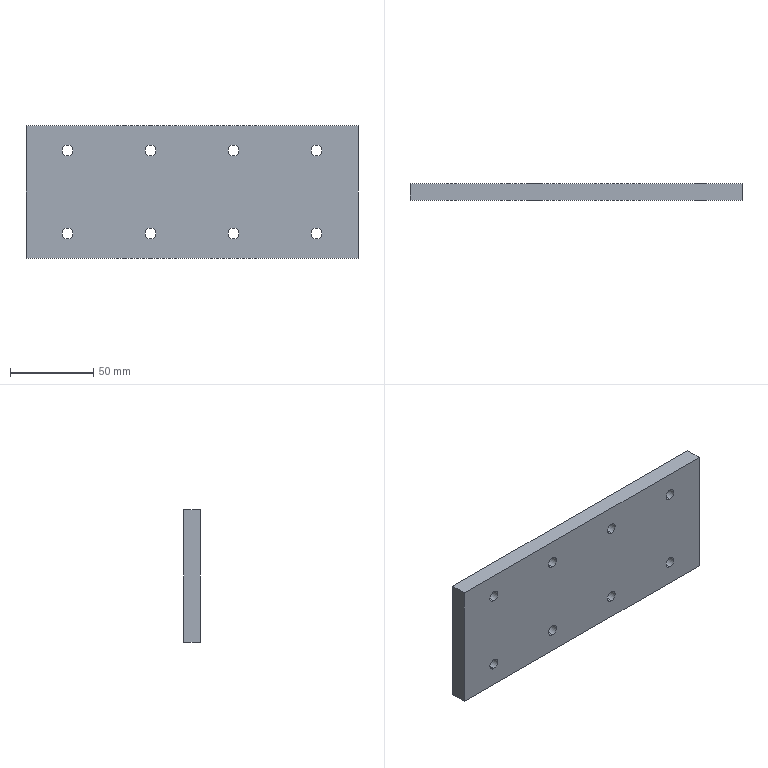Part | SolidWorks | features Extrusion 1, HoleWzd 1 | 1 solid | 22 faces | box 200 x 10 x 80 mm | volume 157263 mm3 | cylinder 16 | plane 6 | commonest cylinder face diameters 6.6 x16
STEP:
#1=CARTESIAN_POINT('',(-25.,0.,-28.3));
#2=VERTEX_POINT('',#1);
#3=CARTESIAN_POINT('',(-25.,0.,-21.7));
#4=VERTEX_POINT('',#3);
#5=CARTESIAN_POINT('',(-25.,0.,-25.));
#6=DIRECTION('',(0.,1.,0.));
#7=DIRECTION('',(0.,0.,1.));
#8=AXIS2_PLACEMENT_3D('',#5,#6,#7);
#9=CIRCLE('',#8,3.3);
#10=EDGE_CURVE('',#2,#4,#9,.T.);
#11=ORIENTED_EDGE('',*,*,#10,.F.);
#12=CARTESIAN_POINT('',(-25.,10.,-28.3));
#13=VERTEX_POINT('',#12);
#14=CARTESIAN_POINT('',(-25.,10.,-28.3));
#15=DIRECTION('',(0.,1.,0.));
#16=VECTOR('',#15,1000.);
#17=LINE('',#14,#16);
#18=EDGE_CURVE('',#2,#13,#17,.T.);
#19=ORIENTED_EDGE('',*,*,#18,.T.);
#20=CARTESIAN_POINT('',(-25.,10.,-21.7));
#21=VERTEX_POINT('',#20);
#22=CARTESIAN_POINT('',(-25.,10.,-25.));
#23=DIRECTION('',(0.,1.,0.));
#24=DIRECTION('',(0.,0.,1.));
#25=AXIS2_PLACEMENT_3D('',#22,#23,#24);
#26=CIRCLE('',#25,3.3);
#27=EDGE_CURVE('',#13,#21,#26,.T.);
#28=ORIENTED_EDGE('',*,*,#27,.T.);
#29=CARTESIAN_POINT('',(-25.,10.,-21.7));
#30=DIRECTION('',(0.,1.,0.));
#31=VECTOR('',#30,1000.);
#32=LINE('',#29,#31);
#33=EDGE_CURVE('',#4,#21,#32,.T.);
#34=ORIENTED_EDGE('',*,*,#33,.F.);
#35=EDGE_LOOP('',(#11,#19,#28,#34));
#36=FACE_OUTER_BOUND('',#35,.T.);
#37=CARTESIAN_POINT('',(-25.,10.,-25.));
#38=DIRECTION('',(0.,1.,0.));
#39=DIRECTION('',(0.,0.,1.));
#40=AXIS2_PLACEMENT_3D('',#37,#38,#39);
#41=CYLINDRICAL_SURFACE('',#40,3.3);
#42=ADVANCED_FACE('',(#36),#41,.F.);
#43=CARTESIAN_POINT('',(25.,0.,-28.3));
#44=VERTEX_POINT('',#43);
#45=CARTESIAN_POINT('',(25.,0.,-21.7));
#46=VERTEX_POINT('',#45);
#47=CARTESIAN_POINT('',(25.,0.,-25.));
#48=DIRECTION('',(0.,1.,0.));
#49=DIRECTION('',(0.,0.,1.));
#50=AXIS2_PLACEMENT_3D('',#47,#48,#49);
#51=CIRCLE('',#50,3.3);
#52=EDGE_CURVE('',#44,#46,#51,.T.);
#53=ORIENTED_EDGE('',*,*,#52,.F.);
#54=CARTESIAN_POINT('',(25.,10.,-28.3));
#55=VERTEX_POINT('',#54);
#56=CARTESIAN_POINT('',(25.,10.,-28.3));
#57=DIRECTION('',(0.,1.,0.));
#58=VECTOR('',#57,1000.);
#59=LINE('',#56,#58);
#60=EDGE_CURVE('',#44,#55,#59,.T.);
#61=ORIENTED_EDGE('',*,*,#60,.T.);
#62=CARTESIAN_POINT('',(25.,10.,-21.7));
#63=VERTEX_POINT('',#62);
#64=CARTESIAN_POINT('',(25.,10.,-25.));
#65=DIRECTION('',(0.,1.,0.));
#66=DIRECTION('',(0.,0.,1.));
#67=AXIS2_PLACEMENT_3D('',#64,#65,#66);
#68=CIRCLE('',#67,3.3);
#69=EDGE_CURVE('',#55,#63,#68,.T.);
#70=ORIENTED_EDGE('',*,*,#69,.T.);
#71=CARTESIAN_POINT('',(25.,10.,-21.7));
#72=DIRECTION('',(0.,1.,0.));
#73=VECTOR('',#72,1000.);
#74=LINE('',#71,#73);
#75=EDGE_CURVE('',#46,#63,#74,.T.);
#76=ORIENTED_EDGE('',*,*,#75,.F.);
#77=EDGE_LOOP('',(#53,#61,#70,#76));
#78=FACE_OUTER_BOUND('',#77,.T.);
#79=CARTESIAN_POINT('',(25.,10.,-25.));
#80=DIRECTION('',(0.,1.,0.));
#81=DIRECTION('',(0.,0.,1.));
#82=AXIS2_PLACEMENT_3D('',#79,#80,#81);
#83=CYLINDRICAL_SURFACE('',#82,3.3);
#84=ADVANCED_FACE('',(#78),#83,.F.);
#85=CARTESIAN_POINT('',(-25.,0.,21.7));
#86=VERTEX_POINT('',#85);
#87=CARTESIAN_POINT('',(-25.,0.,28.3));
#88=VERTEX_POINT('',#87);
#89=CARTESIAN_POINT('',(-25.,0.,25.));
#90=DIRECTION('',(0.,1.,0.));
#91=DIRECTION('',(0.,0.,1.));
#92=AXIS2_PLACEMENT_3D('',#89,#90,#91);
#93=CIRCLE('',#92,3.3);
#94=EDGE_CURVE('',#86,#88,#93,.T.);
#95=ORIENTED_EDGE('',*,*,#94,.F.);
#96=CARTESIAN_POINT('',(-25.,10.,21.7));
#97=VERTEX_POINT('',#96);
#98=CARTESIAN_POINT('',(-25.,10.,21.7));
#99=DIRECTION('',(0.,1.,0.));
#100=VECTOR('',#99,1000.);
#101=LINE('',#98,#100);
#102=EDGE_CURVE('',#86,#97,#101,.T.);
#103=ORIENTED_EDGE('',*,*,#102,.T.);
#104=CARTESIAN_POINT('',(-25.,10.,28.3));
#105=VERTEX_POINT('',#104);
#106=CARTESIAN_POINT('',(-25.,10.,25.));
#107=DIRECTION('',(0.,1.,0.));
#108=DIRECTION('',(0.,0.,1.));
#109=AXIS2_PLACEMENT_3D('',#106,#107,#108);
#110=CIRCLE('',#109,3.3);
#111=EDGE_CURVE('',#97,#105,#110,.T.);
#112=ORIENTED_EDGE('',*,*,#111,.T.);
#113=CARTESIAN_POINT('',(-25.,10.,28.3));
#114=DIRECTION('',(0.,1.,0.));
#115=VECTOR('',#114,1000.);
#116=LINE('',#113,#115);
#117=EDGE_CURVE('',#88,#105,#116,.T.);
#118=ORIENTED_EDGE('',*,*,#117,.F.);
#119=EDGE_LOOP('',(#95,#103,#112,#118));
#120=FACE_OUTER_BOUND('',#119,.T.);
#121=CARTESIAN_POINT('',(-25.,10.,25.));
#122=DIRECTION('',(0.,1.,0.));
#123=DIRECTION('',(0.,0.,1.));
#124=AXIS2_PLACEMENT_3D('',#121,#122,#123);
#125=CYLINDRICAL_SURFACE('',#124,3.3);
#126=ADVANCED_FACE('',(#120),#125,.F.);
#127=CARTESIAN_POINT('',(25.,0.,21.7));
#128=VERTEX_POINT('',#127);
#129=CARTESIAN_POINT('',(25.,0.,28.3));
#130=VERTEX_POINT('',#129);
#131=CARTESIAN_POINT('',(25.,0.,25.));
#132=DIRECTION('',(0.,1.,0.));
#133=DIRECTION('',(0.,0.,1.));
#134=AXIS2_PLACEMENT_3D('',#131,#132,#133);
#135=CIRCLE('',#134,3.3);
#136=EDGE_CURVE('',#128,#130,#135,.T.);
#137=ORIENTED_EDGE('',*,*,#136,.F.);
#138=CARTESIAN_POINT('',(25.,10.,21.7));
#139=VERTEX_POINT('',#138);
#140=CARTESIAN_POINT('',(25.,10.,21.7));
#141=DIRECTION('',(0.,1.,0.));
#142=VECTOR('',#141,1000.);
#143=LINE('',#140,#142);
#144=EDGE_CURVE('',#128,#139,#143,.T.);
#145=ORIENTED_EDGE('',*,*,#144,.T.);
#146=CARTESIAN_POINT('',(25.,10.,28.3));
#147=VERTEX_POINT('',#146);
#148=CARTESIAN_POINT('',(25.,10.,25.));
#149=DIRECTION('',(0.,1.,0.));
#150=DIRECTION('',(0.,0.,1.));
#151=AXIS2_PLACEMENT_3D('',#148,#149,#150);
#152=CIRCLE('',#151,3.3);
#153=EDGE_CURVE('',#139,#147,#152,.T.);
#154=ORIENTED_EDGE('',*,*,#153,.T.);
#155=CARTESIAN_POINT('',(25.,10.,28.3));
#156=DIRECTION('',(0.,1.,0.));
#157=VECTOR('',#156,1000.);
#158=LINE('',#155,#157);
#159=EDGE_CURVE('',#130,#147,#158,.T.);
#160=ORIENTED_EDGE('',*,*,#159,.F.);
#161=EDGE_LOOP('',(#137,#145,#154,#160));
#162=FACE_OUTER_BOUND('',#161,.T.);
#163=CARTESIAN_POINT('',(25.,10.,25.));
#164=DIRECTION('',(0.,1.,0.));
#165=DIRECTION('',(0.,0.,1.));
#166=AXIS2_PLACEMENT_3D('',#163,#164,#165);
#167=CYLINDRICAL_SURFACE('',#166,3.3);
#168=ADVANCED_FACE('',(#162),#167,.F.);
#169=CARTESIAN_POINT('',(-75.,0.,-28.3));
#170=VERTEX_POINT('',#169);
#171=CARTESIAN_POINT('',(-75.,0.,-21.7));
#172=VERTEX_POINT('',#171);
#173=CARTESIAN_POINT('',(-75.,0.,-25.));
#174=DIRECTION('',(0.,1.,0.));
#175=DIRECTION('',(0.,0.,1.));
#176=AXIS2_PLACEMENT_3D('',#173,#174,#175);
#177=CIRCLE('',#176,3.3);
#178=EDGE_CURVE('',#170,#172,#177,.T.);
#179=ORIENTED_EDGE('',*,*,#178,.F.);
#180=CARTESIAN_POINT('',(-75.,10.,-28.3));
#181=VERTEX_POINT('',#180);
#182=CARTESIAN_POINT('',(-75.,10.,-28.3));
#183=DIRECTION('',(0.,1.,0.));
#184=VECTOR('',#183,1000.);
#185=LINE('',#182,#184);
#186=EDGE_CURVE('',#170,#181,#185,.T.);
#187=ORIENTED_EDGE('',*,*,#186,.T.);
#188=CARTESIAN_POINT('',(-75.,10.,-21.7));
#189=VERTEX_POINT('',#188);
#190=CARTESIAN_POINT('',(-75.,10.,-25.));
#191=DIRECTION('',(0.,1.,0.));
#192=DIRECTION('',(0.,0.,1.));
#193=AXIS2_PLACEMENT_3D('',#190,#191,#192);
#194=CIRCLE('',#193,3.3);
#195=EDGE_CURVE('',#181,#189,#194,.T.);
#196=ORIENTED_EDGE('',*,*,#195,.T.);
#197=CARTESIAN_POINT('',(-75.,10.,-21.7));
#198=DIRECTION('',(0.,1.,0.));
#199=VECTOR('',#198,1000.);
#200=LINE('',#197,#199);
#201=EDGE_CURVE('',#172,#189,#200,.T.);
#202=ORIENTED_EDGE('',*,*,#201,.F.);
#203=EDGE_LOOP('',(#179,#187,#196,#202));
#204=FACE_OUTER_BOUND('',#203,.T.);
#205=CARTESIAN_POINT('',(-75.,10.,-25.));
#206=DIRECTION('',(0.,1.,0.));
#207=DIRECTION('',(0.,0.,1.));
#208=AXIS2_PLACEMENT_3D('',#205,#206,#207);
#209=CYLINDRICAL_SURFACE('',#208,3.3);
#210=ADVANCED_FACE('',(#204),#209,.F.);
#211=CARTESIAN_POINT('',(75.,0.,-28.3));
#212=VERTEX_POINT('',#211);
#213=CARTESIAN_POINT('',(75.,0.,-21.7));
#214=VERTEX_POINT('',#213);
#215=CARTESIAN_POINT('',(75.,0.,-25.));
#216=DIRECTION('',(0.,1.,0.));
#217=DIRECTION('',(0.,0.,1.));
#218=AXIS2_PLACEMENT_3D('',#215,#216,#217);
#219=CIRCLE('',#218,3.3);
#220=EDGE_CURVE('',#212,#214,#219,.T.);
#221=ORIENTED_EDGE('',*,*,#220,.F.);
#222=CARTESIAN_POINT('',(75.,10.,-28.3));
#223=VERTEX_POINT('',#222);
#224=CARTESIAN_POINT('',(75.,10.,-28.3));
#225=DIRECTION('',(0.,1.,0.));
#226=VECTOR('',#225,1000.);
#227=LINE('',#224,#226);
#228=EDGE_CURVE('',#212,#223,#227,.T.);
#229=ORIENTED_EDGE('',*,*,#228,.T.);
#230=CARTESIAN_POINT('',(75.,10.,-21.7));
#231=VERTEX_POINT('',#230);
#232=CARTESIAN_POINT('',(75.,10.,-25.));
#233=DIRECTION('',(0.,1.,0.));
#234=DIRECTION('',(0.,0.,1.));
#235=AXIS2_PLACEMENT_3D('',#232,#233,#234);
#236=CIRCLE('',#235,3.3);
#237=EDGE_CURVE('',#223,#231,#236,.T.);
#238=ORIENTED_EDGE('',*,*,#237,.T.);
#239=CARTESIAN_POINT('',(75.,10.,-21.7));
#240=DIRECTION('',(0.,1.,0.));
#241=VECTOR('',#240,1000.);
#242=LINE('',#239,#241);
#243=EDGE_CURVE('',#214,#231,#242,.T.);
#244=ORIENTED_EDGE('',*,*,#243,.F.);
#245=EDGE_LOOP('',(#221,#229,#238,#244));
#246=FACE_OUTER_BOUND('',#245,.T.);
#247=CARTESIAN_POINT('',(75.,10.,-25.));
#248=DIRECTION('',(0.,1.,0.));
#249=DIRECTION('',(0.,0.,1.));
#250=AXIS2_PLACEMENT_3D('',#247,#248,#249);
#251=CYLINDRICAL_SURFACE('',#250,3.3);
#252=ADVANCED_FACE('',(#246),#251,.F.);
#253=CARTESIAN_POINT('',(75.,0.,21.7));
#254=VERTEX_POINT('',#253);
#255=CARTESIAN_POINT('',(75.,0.,28.3));
#256=VERTEX_POINT('',#255);
#257=CARTESIAN_POINT('',(75.,0.,25.));
#258=DIRECTION('',(0.,1.,0.));
#259=DIRECTION('',(0.,0.,1.));
#260=AXIS2_PLACEMENT_3D('',#257,#258,#259);
#261=CIRCLE('',#260,3.3);
#262=EDGE_CURVE('',#254,#256,#261,.T.);
#263=ORIENTED_EDGE('',*,*,#262,.F.);
#264=CARTESIAN_POINT('',(75.,10.,21.7));
#265=VERTEX_POINT('',#264);
#266=CARTESIAN_POINT('',(75.,10.,21.7));
#267=DIRECTION('',(0.,1.,0.));
#268=VECTOR('',#267,1000.);
#269=LINE('',#266,#268);
#270=EDGE_CURVE('',#254,#265,#269,.T.);
#271=ORIENTED_EDGE('',*,*,#270,.T.);
#272=CARTESIAN_POINT('',(75.,10.,28.3));
#273=VERTEX_POINT('',#272);
#274=CARTESIAN_POINT('',(75.,10.,25.));
#275=DIRECTION('',(0.,1.,0.));
#276=DIRECTION('',(0.,0.,1.));
#277=AXIS2_PLACEMENT_3D('',#274,#275,#276);
#278=CIRCLE('',#277,3.3);
#279=EDGE_CURVE('',#265,#273,#278,.T.);
#280=ORIENTED_EDGE('',*,*,#279,.T.);
#281=CARTESIAN_POINT('',(75.,10.,28.3));
#282=DIRECTION('',(0.,1.,0.));
#283=VECTOR('',#282,1000.);
#284=LINE('',#281,#283);
#285=EDGE_CURVE('',#256,#273,#284,.T.);
#286=ORIENTED_EDGE('',*,*,#285,.F.);
#287=EDGE_LOOP('',(#263,#271,#280,#286));
#288=FACE_OUTER_BOUND('',#287,.T.);
#289=CARTESIAN_POINT('',(75.,10.,25.));
#290=DIRECTION('',(0.,1.,0.));
#291=DIRECTION('',(0.,0.,1.));
#292=AXIS2_PLACEMENT_3D('',#289,#290,#291);
#293=CYLINDRICAL_SURFACE('',#292,3.3);
#294=ADVANCED_FACE('',(#288),#293,.F.);
#295=CARTESIAN_POINT('',(-75.,0.,21.7));
#296=VERTEX_POINT('',#295);
#297=CARTESIAN_POINT('',(-75.,0.,28.3));
#298=VERTEX_POINT('',#297);
#299=CARTESIAN_POINT('',(-75.,0.,25.));
#300=DIRECTION('',(0.,1.,0.));
#301=DIRECTION('',(0.,0.,1.));
#302=AXIS2_PLACEMENT_3D('',#299,#300,#301);
#303=CIRCLE('',#302,3.3);
#304=EDGE_CURVE('',#296,#298,#303,.T.);
#305=ORIENTED_EDGE('',*,*,#304,.F.);
#306=CARTESIAN_POINT('',(-75.,10.,21.7));
#307=VERTEX_POINT('',#306);
#308=CARTESIAN_POINT('',(-75.,10.,21.7));
#309=DIRECTION('',(0.,1.,0.));
#310=VECTOR('',#309,1000.);
#311=LINE('',#308,#310);
#312=EDGE_CURVE('',#296,#307,#311,.T.);
#313=ORIENTED_EDGE('',*,*,#312,.T.);
#314=CARTESIAN_POINT('',(-75.,10.,28.3));
#315=VERTEX_POINT('',#314);
#316=CARTESIAN_POINT('',(-75.,10.,25.));
#317=DIRECTION('',(0.,1.,0.));
#318=DIRECTION('',(0.,0.,1.));
#319=AXIS2_PLACEMENT_3D('',#316,#317,#318);
#320=CIRCLE('',#319,3.3);
#321=EDGE_CURVE('',#307,#315,#320,.T.);
#322=ORIENTED_EDGE('',*,*,#321,.T.);
#323=CARTESIAN_POINT('',(-75.,10.,28.3));
#324=DIRECTION('',(0.,1.,0.));
#325=VECTOR('',#324,1000.);
#326=LINE('',#323,#325);
#327=EDGE_CURVE('',#298,#315,#326,.T.);
#328=ORIENTED_EDGE('',*,*,#327,.F.);
#329=EDGE_LOOP('',(#305,#313,#322,#328));
#330=FACE_OUTER_BOUND('',#329,.T.);
#331=CARTESIAN_POINT('',(-75.,10.,25.));
#332=DIRECTION('',(0.,1.,0.));
#333=DIRECTION('',(0.,0.,1.));
#334=AXIS2_PLACEMENT_3D('',#331,#332,#333);
#335=CYLINDRICAL_SURFACE('',#334,3.3);
#336=ADVANCED_FACE('',(#330),#335,.F.);
#337=CARTESIAN_POINT('',(100.,0.,40.));
#338=VERTEX_POINT('',#337);
#339=CARTESIAN_POINT('',(100.,0.,-40.));
#340=VERTEX_POINT('',#339);
#341=CARTESIAN_POINT('',(100.,0.,-40.));
#342=DIRECTION('',(0.,0.,-1.));
#343=VECTOR('',#342,1000.);
#344=LINE('',#341,#343);
#345=EDGE_CURVE('',#338,#340,#344,.T.);
#346=ORIENTED_EDGE('',*,*,#345,.T.);
#347=CARTESIAN_POINT('',(100.,10.,-40.));
#348=VERTEX_POINT('',#347);
#349=CARTESIAN_POINT('',(100.,10.,-40.));
#350=DIRECTION('',(0.,-1.,0.));
#351=VECTOR('',#350,1000.);
#352=LINE('',#349,#351);
#353=EDGE_CURVE('',#348,#340,#352,.T.);
#354=ORIENTED_EDGE('',*,*,#353,.F.);
#355=CARTESIAN_POINT('',(100.,10.,40.));
#356=VERTEX_POINT('',#355);
#357=CARTESIAN_POINT('',(100.,10.,-40.));
#358=DIRECTION('',(0.,0.,-1.));
#359=VECTOR('',#358,1000.);
#360=LINE('',#357,#359);
#361=EDGE_CURVE('',#356,#348,#360,.T.);
#362=ORIENTED_EDGE('',*,*,#361,.F.);
#363=CARTESIAN_POINT('',(100.,10.,40.));
#364=DIRECTION('',(0.,-1.,0.));
#365=VECTOR('',#364,1000.);
#366=LINE('',#363,#365);
#367=EDGE_CURVE('',#356,#338,#366,.T.);
#368=ORIENTED_EDGE('',*,*,#367,.T.);
#369=EDGE_LOOP('',(#346,#354,#362,#368));
#370=FACE_OUTER_BOUND('',#369,.T.);
#371=CARTESIAN_POINT('',(100.,10.,-40.));
#372=DIRECTION('',(-1.,0.,0.));
#373=DIRECTION('',(0.,0.,1.));
#374=AXIS2_PLACEMENT_3D('',#371,#372,#373);
#375=PLANE('',#374);
#376=ADVANCED_FACE('',(#370),#375,.F.);
#377=CARTESIAN_POINT('',(-100.,0.,-40.));
#378=VERTEX_POINT('',#377);
#379=CARTESIAN_POINT('',(-100.,0.,-40.));
#380=DIRECTION('',(-1.,0.,0.));
#381=VECTOR('',#380,1000.);
#382=LINE('',#379,#381);
#383=EDGE_CURVE('',#340,#378,#382,.T.);
#384=ORIENTED_EDGE('',*,*,#383,.T.);
#385=CARTESIAN_POINT('',(-100.,10.,-40.));
#386=VERTEX_POINT('',#385);
#387=CARTESIAN_POINT('',(-100.,10.,-40.));
#388=DIRECTION('',(0.,-1.,0.));
#389=VECTOR('',#388,1000.);
#390=LINE('',#387,#389);
#391=EDGE_CURVE('',#386,#378,#390,.T.);
#392=ORIENTED_EDGE('',*,*,#391,.F.);
#393=CARTESIAN_POINT('',(-100.,10.,-40.));
#394=DIRECTION('',(-1.,0.,0.));
#395=VECTOR('',#394,1000.);
#396=LINE('',#393,#395);
#397=EDGE_CURVE('',#348,#386,#396,.T.);
#398=ORIENTED_EDGE('',*,*,#397,.F.);
#399=ORIENTED_EDGE('',*,*,#353,.T.);
#400=EDGE_LOOP('',(#384,#392,#398,#399));
#401=FACE_OUTER_BOUND('',#400,.T.);
#402=CARTESIAN_POINT('',(-100.,10.,-40.));
#403=DIRECTION('',(0.,0.,1.));
#404=DIRECTION('',(1.,0.,0.));
#405=AXIS2_PLACEMENT_3D('',#402,#403,#404);
#406=PLANE('',#405);
#407=ADVANCED_FACE('',(#401),#406,.F.);
#408=CARTESIAN_POINT('',(-100.,0.,40.));
#409=VERTEX_POINT('',#408);
#410=CARTESIAN_POINT('',(-100.,0.,-40.));
#411=DIRECTION('',(0.,0.,1.));
#412=VECTOR('',#411,1000.);
#413=LINE('',#410,#412);
#414=EDGE_CURVE('',#378,#409,#413,.T.);
#415=ORIENTED_EDGE('',*,*,#414,.T.);
#416=CARTESIAN_POINT('',(-100.,10.,40.));
#417=VERTEX_POINT('',#416);
#418=CARTESIAN_POINT('',(-100.,10.,40.));
#419=DIRECTION('',(0.,-1.,0.));
#420=VECTOR('',#419,1000.);
#421=LINE('',#418,#420);
#422=EDGE_CURVE('',#417,#409,#421,.T.);
#423=ORIENTED_EDGE('',*,*,#422,.F.);
#424=CARTESIAN_POINT('',(-100.,10.,-40.));
#425=DIRECTION('',(0.,0.,1.));
#426=VECTOR('',#425,1000.);
#427=LINE('',#424,#426);
#428=EDGE_CURVE('',#386,#417,#427,.T.);
#429=ORIENTED_EDGE('',*,*,#428,.F.);
#430=ORIENTED_EDGE('',*,*,#391,.T.);
#431=EDGE_LOOP('',(#415,#423,#429,#430));
#432=FACE_OUTER_BOUND('',#431,.T.);
#433=CARTESIAN_POINT('',(-100.,10.,-40.));
#434=DIRECTION('',(1.,0.,0.));
#435=DIRECTION('',(0.,0.,-1.));
#436=AXIS2_PLACEMENT_3D('',#433,#434,#435);
#437=PLANE('',#436);
#438=ADVANCED_FACE('',(#432),#437,.F.);
#439=CARTESIAN_POINT('',(-100.,0.,40.));
#440=DIRECTION('',(1.,0.,0.));
#441=VECTOR('',#440,1000.);
#442=LINE('',#439,#441);
#443=EDGE_CURVE('',#409,#338,#442,.T.);
#444=ORIENTED_EDGE('',*,*,#443,.T.);
#445=ORIENTED_EDGE('',*,*,#367,.F.);
#446=CARTESIAN_POINT('',(-100.,10.,40.));
#447=DIRECTION('',(1.,0.,0.));
#448=VECTOR('',#447,1000.);
#449=LINE('',#446,#448);
#450=EDGE_CURVE('',#417,#356,#449,.T.);
#451=ORIENTED_EDGE('',*,*,#450,.F.);
#452=ORIENTED_EDGE('',*,*,#422,.T.);
#453=EDGE_LOOP('',(#444,#445,#451,#452));
#454=FACE_OUTER_BOUND('',#453,.T.);
#455=CARTESIAN_POINT('',(-100.,10.,40.));
#456=DIRECTION('',(0.,0.,-1.));
#457=DIRECTION('',(-1.,0.,0.));
#458=AXIS2_PLACEMENT_3D('',#455,#456,#457);
#459=PLANE('',#458);
#460=ADVANCED_FACE('',(#454),#459,.F.);
#461=CARTESIAN_POINT('',(-25.,10.,-25.));
#462=DIRECTION('',(0.,1.,0.));
#463=DIRECTION('',(0.,0.,1.));
#464=AXIS2_PLACEMENT_3D('',#461,#462,#463);
#465=CIRCLE('',#464,3.3);
#466=EDGE_CURVE('',#21,#13,#465,.T.);
#467=ORIENTED_EDGE('',*,*,#466,.F.);
#468=ORIENTED_EDGE('',*,*,#27,.F.);
#469=EDGE_LOOP('',(#467,#468));
#470=FACE_BOUND('',#469,.T.);
#471=CARTESIAN_POINT('',(25.,10.,-25.));
#472=DIRECTION('',(0.,1.,0.));
#473=DIRECTION('',(0.,0.,1.));
#474=AXIS2_PLACEMENT_3D('',#471,#472,#473);
#475=CIRCLE('',#474,3.3);
#476=EDGE_CURVE('',#63,#55,#475,.T.);
#477=ORIENTED_EDGE('',*,*,#476,.F.);
#478=ORIENTED_EDGE('',*,*,#69,.F.);
#479=EDGE_LOOP('',(#477,#478));
#480=FACE_BOUND('',#479,.T.);
#481=CARTESIAN_POINT('',(-25.,10.,25.));
#482=DIRECTION('',(0.,1.,0.));
#483=DIRECTION('',(0.,0.,1.));
#484=AXIS2_PLACEMENT_3D('',#481,#482,#483);
#485=CIRCLE('',#484,3.3);
#486=EDGE_CURVE('',#105,#97,#485,.T.);
#487=ORIENTED_EDGE('',*,*,#486,.F.);
#488=ORIENTED_EDGE('',*,*,#111,.F.);
#489=EDGE_LOOP('',(#487,#488));
#490=FACE_BOUND('',#489,.T.);
#491=CARTESIAN_POINT('',(25.,10.,25.));
#492=DIRECTION('',(0.,1.,0.));
#493=DIRECTION('',(0.,0.,1.));
#494=AXIS2_PLACEMENT_3D('',#491,#492,#493);
#495=CIRCLE('',#494,3.3);
#496=EDGE_CURVE('',#147,#139,#495,.T.);
#497=ORIENTED_EDGE('',*,*,#496,.F.);
#498=ORIENTED_EDGE('',*,*,#153,.F.);
#499=EDGE_LOOP('',(#497,#498));
#500=FACE_BOUND('',#499,.T.);
#501=CARTESIAN_POINT('',(-75.,10.,-25.));
#502=DIRECTION('',(0.,1.,0.));
#503=DIRECTION('',(0.,0.,1.));
#504=AXIS2_PLACEMENT_3D('',#501,#502,#503);
#505=CIRCLE('',#504,3.3);
#506=EDGE_CURVE('',#189,#181,#505,.T.);
#507=ORIENTED_EDGE('',*,*,#506,.F.);
#508=ORIENTED_EDGE('',*,*,#195,.F.);
#509=EDGE_LOOP('',(#507,#508));
#510=FACE_BOUND('',#509,.T.);
#511=CARTESIAN_POINT('',(75.,10.,-25.));
#512=DIRECTION('',(0.,1.,0.));
#513=DIRECTION('',(0.,0.,1.));
#514=AXIS2_PLACEMENT_3D('',#511,#512,#513);
#515=CIRCLE('',#514,3.3);
#516=EDGE_CURVE('',#231,#223,#515,.T.);
#517=ORIENTED_EDGE('',*,*,#516,.F.);
#518=ORIENTED_EDGE('',*,*,#237,.F.);
#519=EDGE_LOOP('',(#517,#518));
#520=FACE_BOUND('',#519,.T.);
#521=CARTESIAN_POINT('',(75.,10.,25.));
#522=DIRECTION('',(0.,1.,0.));
#523=DIRECTION('',(0.,0.,1.));
#524=AXIS2_PLACEMENT_3D('',#521,#522,#523);
#525=CIRCLE('',#524,3.3);
#526=EDGE_CURVE('',#273,#265,#525,.T.);
#527=ORIENTED_EDGE('',*,*,#526,.F.);
#528=ORIENTED_EDGE('',*,*,#279,.F.);
#529=EDGE_LOOP('',(#527,#528));
#530=FACE_BOUND('',#529,.T.);
#531=CARTESIAN_POINT('',(-75.,10.,25.));
#532=DIRECTION('',(0.,1.,0.));
#533=DIRECTION('',(0.,0.,1.));
#534=AXIS2_PLACEMENT_3D('',#531,#532,#533);
#535=CIRCLE('',#534,3.3);
#536=EDGE_CURVE('',#315,#307,#535,.T.);
#537=ORIENTED_EDGE('',*,*,#536,.F.);
#538=ORIENTED_EDGE('',*,*,#321,.F.);
#539=EDGE_LOOP('',(#537,#538));
#540=FACE_BOUND('',#539,.T.);
#541=ORIENTED_EDGE('',*,*,#361,.T.);
#542=ORIENTED_EDGE('',*,*,#397,.T.);
#543=ORIENTED_EDGE('',*,*,#428,.T.);
#544=ORIENTED_EDGE('',*,*,#450,.T.);
#545=EDGE_LOOP('',(#541,#542,#543,#544));
#546=FACE_OUTER_BOUND('',#545,.T.);
#547=CARTESIAN_POINT('',(0.,10.,0.));
#548=DIRECTION('',(0.,1.,0.));
#549=DIRECTION('',(0.,0.,1.));
#550=AXIS2_PLACEMENT_3D('',#547,#548,#549);
#551=PLANE('',#550);
#552=ADVANCED_FACE('',(#470,#480,#490,#500,#510,#520,#530,#540,#546),#551,.T.);
#553=CARTESIAN_POINT('',(-25.,0.,-25.));
#554=DIRECTION('',(0.,1.,0.));
#555=DIRECTION('',(0.,0.,1.));
#556=AXIS2_PLACEMENT_3D('',#553,#554,#555);
#557=CIRCLE('',#556,3.3);
#558=EDGE_CURVE('',#4,#2,#557,.T.);
#559=ORIENTED_EDGE('',*,*,#558,.T.);
#560=ORIENTED_EDGE('',*,*,#10,.T.);
#561=EDGE_LOOP('',(#559,#560));
#562=FACE_BOUND('',#561,.T.);
#563=CARTESIAN_POINT('',(25.,0.,-25.));
#564=DIRECTION('',(0.,1.,0.));
#565=DIRECTION('',(0.,0.,1.));
#566=AXIS2_PLACEMENT_3D('',#563,#564,#565);
#567=CIRCLE('',#566,3.3);
#568=EDGE_CURVE('',#46,#44,#567,.T.);
#569=ORIENTED_EDGE('',*,*,#568,.T.);
#570=ORIENTED_EDGE('',*,*,#52,.T.);
#571=EDGE_LOOP('',(#569,#570));
#572=FACE_BOUND('',#571,.T.);
#573=CARTESIAN_POINT('',(-25.,0.,25.));
#574=DIRECTION('',(0.,1.,0.));
#575=DIRECTION('',(0.,0.,1.));
#576=AXIS2_PLACEMENT_3D('',#573,#574,#575);
#577=CIRCLE('',#576,3.3);
#578=EDGE_CURVE('',#88,#86,#577,.T.);
#579=ORIENTED_EDGE('',*,*,#578,.T.);
#580=ORIENTED_EDGE('',*,*,#94,.T.);
#581=EDGE_LOOP('',(#579,#580));
#582=FACE_BOUND('',#581,.T.);
#583=CARTESIAN_POINT('',(25.,0.,25.));
#584=DIRECTION('',(0.,1.,0.));
#585=DIRECTION('',(0.,0.,1.));
#586=AXIS2_PLACEMENT_3D('',#583,#584,#585);
#587=CIRCLE('',#586,3.3);
#588=EDGE_CURVE('',#130,#128,#587,.T.);
#589=ORIENTED_EDGE('',*,*,#588,.T.);
#590=ORIENTED_EDGE('',*,*,#136,.T.);
#591=EDGE_LOOP('',(#589,#590));
#592=FACE_BOUND('',#591,.T.);
#593=CARTESIAN_POINT('',(-75.,0.,-25.));
#594=DIRECTION('',(0.,1.,0.));
#595=DIRECTION('',(0.,0.,1.));
#596=AXIS2_PLACEMENT_3D('',#593,#594,#595);
#597=CIRCLE('',#596,3.3);
#598=EDGE_CURVE('',#172,#170,#597,.T.);
#599=ORIENTED_EDGE('',*,*,#598,.T.);
#600=ORIENTED_EDGE('',*,*,#178,.T.);
#601=EDGE_LOOP('',(#599,#600));
#602=FACE_BOUND('',#601,.T.);
#603=CARTESIAN_POINT('',(75.,0.,-25.));
#604=DIRECTION('',(0.,1.,0.));
#605=DIRECTION('',(0.,0.,1.));
#606=AXIS2_PLACEMENT_3D('',#603,#604,#605);
#607=CIRCLE('',#606,3.3);
#608=EDGE_CURVE('',#214,#212,#607,.T.);
#609=ORIENTED_EDGE('',*,*,#608,.T.);
#610=ORIENTED_EDGE('',*,*,#220,.T.);
#611=EDGE_LOOP('',(#609,#610));
#612=FACE_BOUND('',#611,.T.);
#613=CARTESIAN_POINT('',(75.,0.,25.));
#614=DIRECTION('',(0.,1.,0.));
#615=DIRECTION('',(0.,0.,1.));
#616=AXIS2_PLACEMENT_3D('',#613,#614,#615);
#617=CIRCLE('',#616,3.3);
#618=EDGE_CURVE('',#256,#254,#617,.T.);
#619=ORIENTED_EDGE('',*,*,#618,.T.);
#620=ORIENTED_EDGE('',*,*,#262,.T.);
#621=EDGE_LOOP('',(#619,#620));
#622=FACE_BOUND('',#621,.T.);
#623=CARTESIAN_POINT('',(-75.,0.,25.));
#624=DIRECTION('',(0.,1.,0.));
#625=DIRECTION('',(0.,0.,1.));
#626=AXIS2_PLACEMENT_3D('',#623,#624,#625);
#627=CIRCLE('',#626,3.3);
#628=EDGE_CURVE('',#298,#296,#627,.T.);
#629=ORIENTED_EDGE('',*,*,#628,.T.);
#630=ORIENTED_EDGE('',*,*,#304,.T.);
#631=EDGE_LOOP('',(#629,#630));
#632=FACE_BOUND('',#631,.T.);
#633=ORIENTED_EDGE('',*,*,#345,.F.);
#634=ORIENTED_EDGE('',*,*,#443,.F.);
#635=ORIENTED_EDGE('',*,*,#414,.F.);
#636=ORIENTED_EDGE('',*,*,#383,.F.);
#637=EDGE_LOOP('',(#633,#634,#635,#636));
#638=FACE_OUTER_BOUND('',#637,.T.);
#639=CARTESIAN_POINT('',(0.,0.,0.));
#640=DIRECTION('',(0.,1.,0.));
#641=DIRECTION('',(0.,0.,1.));
#642=AXIS2_PLACEMENT_3D('',#639,#640,#641);
#643=PLANE('',#642);
#644=ADVANCED_FACE('',(#562,#572,#582,#592,#602,#612,#622,#632,#638),#643,.F.);
#645=ORIENTED_EDGE('',*,*,#312,.F.);
#646=ORIENTED_EDGE('',*,*,#628,.F.);
#647=ORIENTED_EDGE('',*,*,#327,.T.);
#648=ORIENTED_EDGE('',*,*,#536,.T.);
#649=EDGE_LOOP('',(#645,#646,#647,#648));
#650=FACE_OUTER_BOUND('',#649,.T.);
#651=CARTESIAN_POINT('',(-75.,10.,25.));
#652=DIRECTION('',(0.,1.,0.));
#653=DIRECTION('',(0.,0.,1.));
#654=AXIS2_PLACEMENT_3D('',#651,#652,#653);
#655=CYLINDRICAL_SURFACE('',#654,3.3);
#656=ADVANCED_FACE('',(#650),#655,.F.);
#657=ORIENTED_EDGE('',*,*,#270,.F.);
#658=ORIENTED_EDGE('',*,*,#618,.F.);
#659=ORIENTED_EDGE('',*,*,#285,.T.);
#660=ORIENTED_EDGE('',*,*,#526,.T.);
#661=EDGE_LOOP('',(#657,#658,#659,#660));
#662=FACE_OUTER_BOUND('',#661,.T.);
#663=CARTESIAN_POINT('',(75.,10.,25.));
#664=DIRECTION('',(0.,1.,0.));
#665=DIRECTION('',(0.,0.,1.));
#666=AXIS2_PLACEMENT_3D('',#663,#664,#665);
#667=CYLINDRICAL_SURFACE('',#666,3.3);
#668=ADVANCED_FACE('',(#662),#667,.F.);
#669=ORIENTED_EDGE('',*,*,#228,.F.);
#670=ORIENTED_EDGE('',*,*,#608,.F.);
#671=ORIENTED_EDGE('',*,*,#243,.T.);
#672=ORIENTED_EDGE('',*,*,#516,.T.);
#673=EDGE_LOOP('',(#669,#670,#671,#672));
#674=FACE_OUTER_BOUND('',#673,.T.);
#675=CARTESIAN_POINT('',(75.,10.,-25.));
#676=DIRECTION('',(0.,1.,0.));
#677=DIRECTION('',(0.,0.,1.));
#678=AXIS2_PLACEMENT_3D('',#675,#676,#677);
#679=CYLINDRICAL_SURFACE('',#678,3.3);
#680=ADVANCED_FACE('',(#674),#679,.F.);
#681=ORIENTED_EDGE('',*,*,#186,.F.);
#682=ORIENTED_EDGE('',*,*,#598,.F.);
#683=ORIENTED_EDGE('',*,*,#201,.T.);
#684=ORIENTED_EDGE('',*,*,#506,.T.);
#685=EDGE_LOOP('',(#681,#682,#683,#684));
#686=FACE_OUTER_BOUND('',#685,.T.);
#687=CARTESIAN_POINT('',(-75.,10.,-25.));
#688=DIRECTION('',(0.,1.,0.));
#689=DIRECTION('',(0.,0.,1.));
#690=AXIS2_PLACEMENT_3D('',#687,#688,#689);
#691=CYLINDRICAL_SURFACE('',#690,3.3);
#692=ADVANCED_FACE('',(#686),#691,.F.);
#693=ORIENTED_EDGE('',*,*,#144,.F.);
#694=ORIENTED_EDGE('',*,*,#588,.F.);
#695=ORIENTED_EDGE('',*,*,#159,.T.);
#696=ORIENTED_EDGE('',*,*,#496,.T.);
#697=EDGE_LOOP('',(#693,#694,#695,#696));
#698=FACE_OUTER_BOUND('',#697,.T.);
#699=CARTESIAN_POINT('',(25.,10.,25.));
#700=DIRECTION('',(0.,1.,0.));
#701=DIRECTION('',(0.,0.,1.));
#702=AXIS2_PLACEMENT_3D('',#699,#700,#701);
#703=CYLINDRICAL_SURFACE('',#702,3.3);
#704=ADVANCED_FACE('',(#698),#703,.F.);
#705=ORIENTED_EDGE('',*,*,#102,.F.);
#706=ORIENTED_EDGE('',*,*,#578,.F.);
#707=ORIENTED_EDGE('',*,*,#117,.T.);
#708=ORIENTED_EDGE('',*,*,#486,.T.);
#709=EDGE_LOOP('',(#705,#706,#707,#708));
#710=FACE_OUTER_BOUND('',#709,.T.);
#711=CARTESIAN_POINT('',(-25.,10.,25.));
#712=DIRECTION('',(0.,1.,0.));
#713=DIRECTION('',(0.,0.,1.));
#714=AXIS2_PLACEMENT_3D('',#711,#712,#713);
#715=CYLINDRICAL_SURFACE('',#714,3.3);
#716=ADVANCED_FACE('',(#710),#715,.F.);
#717=ORIENTED_EDGE('',*,*,#60,.F.);
#718=ORIENTED_EDGE('',*,*,#568,.F.);
#719=ORIENTED_EDGE('',*,*,#75,.T.);
#720=ORIENTED_EDGE('',*,*,#476,.T.);
#721=EDGE_LOOP('',(#717,#718,#719,#720));
#722=FACE_OUTER_BOUND('',#721,.T.);
#723=CARTESIAN_POINT('',(25.,10.,-25.));
#724=DIRECTION('',(0.,1.,0.));
#725=DIRECTION('',(0.,0.,1.));
#726=AXIS2_PLACEMENT_3D('',#723,#724,#725);
#727=CYLINDRICAL_SURFACE('',#726,3.3);
#728=ADVANCED_FACE('',(#722),#727,.F.);
#729=ORIENTED_EDGE('',*,*,#18,.F.);
#730=ORIENTED_EDGE('',*,*,#558,.F.);
#731=ORIENTED_EDGE('',*,*,#33,.T.);
#732=ORIENTED_EDGE('',*,*,#466,.T.);
#733=EDGE_LOOP('',(#729,#730,#731,#732));
#734=FACE_OUTER_BOUND('',#733,.T.);
#735=CARTESIAN_POINT('',(-25.,10.,-25.));
#736=DIRECTION('',(0.,1.,0.));
#737=DIRECTION('',(0.,0.,1.));
#738=AXIS2_PLACEMENT_3D('',#735,#736,#737);
#739=CYLINDRICAL_SURFACE('',#738,3.3);
#740=ADVANCED_FACE('',(#734),#739,.F.);
#741=CLOSED_SHELL('',(#42,#84,#126,#168,#210,#252,#294,#336,#376,#407,#438,#460,#552,#644,#656,#668,#680,#692,#704,#716,#728,#740));
#742=MANIFOLD_SOLID_BREP('',#741);
#743=CARTESIAN_POINT('',(0.,0.,0.));
#744=DIRECTION('',(0.,0.,1.));
#745=DIRECTION('',(1.,0.,0.));
#746=AXIS2_PLACEMENT_3D('',#743,#744,#745);
#747=(LENGTH_UNIT()NAMED_UNIT(*)SI_UNIT(.MILLI.,.METRE.));
#748=UNCERTAINTY_MEASURE_WITH_UNIT(LENGTH_MEASURE(0.00001),#747,'','');
#749=(NAMED_UNIT(*)PLANE_ANGLE_UNIT()SI_UNIT($,.RADIAN.));
#750=(NAMED_UNIT(*)SI_UNIT($,.STERADIAN.)SOLID_ANGLE_UNIT());
#751=(GEOMETRIC_REPRESENTATION_CONTEXT(3)GLOBAL_UNCERTAINTY_ASSIGNED_CONTEXT((#748))GLOBAL_UNIT_ASSIGNED_CONTEXT((#747,#749,#750))REPRESENTATION_CONTEXT('',''));
#752=ADVANCED_BREP_SHAPE_REPRESENTATION('',(#742,#746),#751);